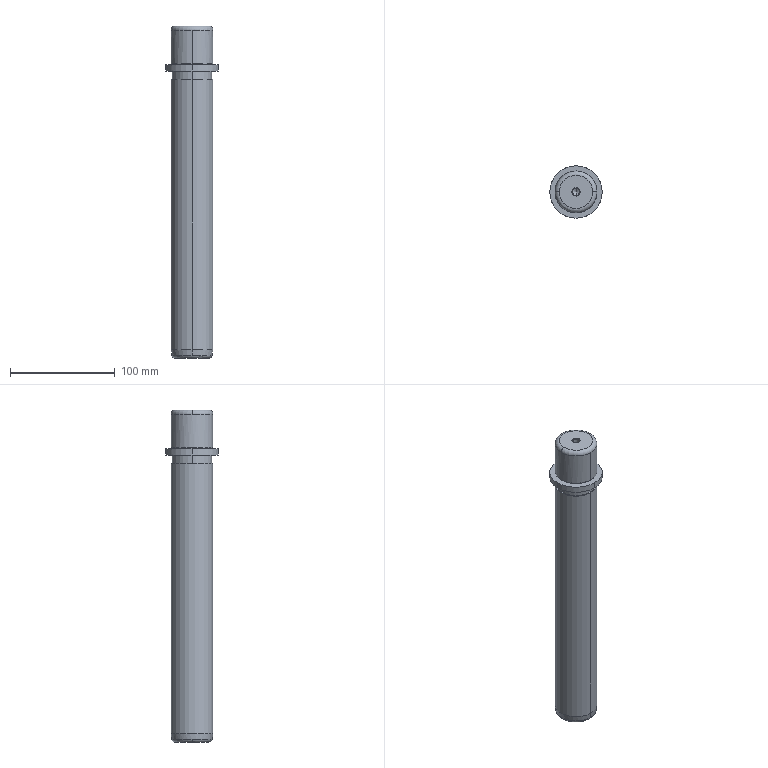Part | CATIA | 1 solid | 37 faces | box 50 x 50 x 317 mm | volume 398728 mm3 | cylinder 19 | cone 8 | plane 6 | torus 4 | commonest cylinder face diameters 38 x7 6.647 x4 40 x4 50 x4
STEP:
#1=CARTESIAN_POINT('',(0.,-3.323,16.609));
#2=VERTEX_POINT('',#1);
#3=CARTESIAN_POINT('',(0.,0.,14.691));
#4=VERTEX_POINT('',#3);
#5=CARTESIAN_POINT('',(0.,-433013.533,250015.17));
#6=DIRECTION('',(0.,-0.866,0.5));
#7=VECTOR('',#6,1.);
#8=LINE('',#5,#7);
#9=EDGE_CURVE('',#2,#4,#8,.F.);
#10=ORIENTED_EDGE('',*,*,#9,.T.);
#11=CARTESIAN_POINT('',(0.,3.323,16.609));
#12=VERTEX_POINT('',#11);
#13=CARTESIAN_POINT('',(0.,433013.533,250015.17));
#14=DIRECTION('',(0.,0.866,0.5));
#15=VECTOR('',#14,1.);
#16=LINE('',#13,#15);
#17=EDGE_CURVE('',#4,#12,#16,.T.);
#18=ORIENTED_EDGE('',*,*,#17,.T.);
#19=CARTESIAN_POINT('',(0.,0.,16.609));
#20=DIRECTION('',(0.,0.,1.));
#21=AXIS2_PLACEMENT_3D('',#19,#20,$);
#22=CIRCLE('',#21,3.323);
#23=EDGE_CURVE('',#12,#2,#22,.T.);
#24=ORIENTED_EDGE('',*,*,#23,.T.);
#25=EDGE_LOOP('',(#10,#18,#24));
#26=FACE_OUTER_BOUND('',#25,.T.);
#27=CARTESIAN_POINT('',(0.,0.,15.65));
#28=DIRECTION('',(0.,0.,1.));
#29=DIRECTION('',(0.,1.,0.));
#30=AXIS2_PLACEMENT_3D('',#27,#28,#29);
#31=CONICAL_SURFACE('',#30,1.662,1.047);
#32=ADVANCED_FACE('',(#26),#31,.F.);
#33=ORIENTED_EDGE('',*,*,#9,.F.);
#34=CARTESIAN_POINT('',(0.,0.,16.609));
#35=DIRECTION('',(0.,0.,1.));
#36=AXIS2_PLACEMENT_3D('',#34,#35,$);
#37=CIRCLE('',#36,3.323);
#38=EDGE_CURVE('',#2,#12,#37,.T.);
#39=ORIENTED_EDGE('',*,*,#38,.T.);
#40=ORIENTED_EDGE('',*,*,#17,.F.);
#41=EDGE_LOOP('',(#33,#39,#40));
#42=FACE_OUTER_BOUND('',#41,.T.);
#43=CARTESIAN_POINT('',(0.,0.,15.65));
#44=DIRECTION('',(0.,0.,1.));
#45=DIRECTION('',(0.,-1.,0.));
#46=AXIS2_PLACEMENT_3D('',#43,#44,#45);
#47=CONICAL_SURFACE('',#46,1.662,1.047);
#48=ADVANCED_FACE('',(#42),#47,.F.);
#49=CARTESIAN_POINT('',(0.,3.324,36.324));
#50=VERTEX_POINT('',#49);
#51=CARTESIAN_POINT('',(0.,3.324,26.466));
#52=DIRECTION('',(0.,0.,-1.));
#53=VECTOR('',#52,1.);
#54=LINE('',#51,#53);
#55=EDGE_CURVE('',#12,#50,#54,.F.);
#56=ORIENTED_EDGE('',*,*,#55,.T.);
#57=CARTESIAN_POINT('',(0.,-3.324,36.324));
#58=VERTEX_POINT('',#57);
#59=CARTESIAN_POINT('',(0.,0.,36.324));
#60=DIRECTION('',(0.,0.,-1.));
#61=AXIS2_PLACEMENT_3D('',#59,#60,$);
#62=CIRCLE('',#61,3.324);
#63=EDGE_CURVE('',#50,#58,#62,.F.);
#64=ORIENTED_EDGE('',*,*,#63,.T.);
#65=CARTESIAN_POINT('',(0.,-3.324,26.466));
#66=DIRECTION('',(0.,0.,-1.));
#67=VECTOR('',#66,1.);
#68=LINE('',#65,#67);
#69=EDGE_CURVE('',#58,#2,#68,.T.);
#70=ORIENTED_EDGE('',*,*,#69,.T.);
#71=ORIENTED_EDGE('',*,*,#23,.F.);
#72=EDGE_LOOP('',(#56,#64,#70,#71));
#73=FACE_OUTER_BOUND('',#72,.T.);
#74=CARTESIAN_POINT('',(0.,0.,26.466));
#75=DIRECTION('',(0.,0.,-1.));
#76=DIRECTION('',(0.,-1.,0.));
#77=AXIS2_PLACEMENT_3D('',#74,#75,#76);
#78=CYLINDRICAL_SURFACE('',#77,3.324);
#79=ADVANCED_FACE('',(#73),#78,.F.);
#80=ORIENTED_EDGE('',*,*,#55,.F.);
#81=ORIENTED_EDGE('',*,*,#38,.F.);
#82=ORIENTED_EDGE('',*,*,#69,.F.);
#83=CARTESIAN_POINT('',(0.,0.,36.324));
#84=DIRECTION('',(0.,0.,-1.));
#85=AXIS2_PLACEMENT_3D('',#83,#84,$);
#86=CIRCLE('',#85,3.324);
#87=EDGE_CURVE('',#58,#50,#86,.F.);
#88=ORIENTED_EDGE('',*,*,#87,.T.);
#89=EDGE_LOOP('',(#80,#81,#82,#88));
#90=FACE_OUTER_BOUND('',#89,.T.);
#91=CARTESIAN_POINT('',(0.,0.,26.466));
#92=DIRECTION('',(0.,0.,-1.));
#93=DIRECTION('',(0.,1.,0.));
#94=AXIS2_PLACEMENT_3D('',#91,#92,#93);
#95=CYLINDRICAL_SURFACE('',#94,3.324);
#96=ADVANCED_FACE('',(#90),#95,.F.);
#97=CARTESIAN_POINT('',(0.,4.,37.));
#98=VERTEX_POINT('',#97);
#99=CARTESIAN_POINT('',(0.,353555.221,353588.221));
#100=DIRECTION('',(0.,0.7071,0.7071));
#101=VECTOR('',#100,1.);
#102=LINE('',#99,#101);
#103=EDGE_CURVE('',#50,#98,#102,.T.);
#104=ORIENTED_EDGE('',*,*,#103,.T.);
#105=CARTESIAN_POINT('',(0.,-4.,37.));
#106=VERTEX_POINT('',#105);
#107=CARTESIAN_POINT('',(0.,0.,37.));
#108=DIRECTION('',(0.,0.,1.));
#109=AXIS2_PLACEMENT_3D('',#107,#108,$);
#110=CIRCLE('',#109,4.);
#111=EDGE_CURVE('',#98,#106,#110,.T.);
#112=ORIENTED_EDGE('',*,*,#111,.T.);
#113=CARTESIAN_POINT('',(0.,-353555.221,353588.221));
#114=DIRECTION('',(0.,-0.7071,0.7071));
#115=VECTOR('',#114,1.);
#116=LINE('',#113,#115);
#117=EDGE_CURVE('',#106,#58,#116,.F.);
#118=ORIENTED_EDGE('',*,*,#117,.T.);
#119=ORIENTED_EDGE('',*,*,#63,.F.);
#120=EDGE_LOOP('',(#104,#112,#118,#119));
#121=FACE_OUTER_BOUND('',#120,.T.);
#122=CARTESIAN_POINT('',(0.,0.,36.662));
#123=DIRECTION('',(0.,0.,1.));
#124=DIRECTION('',(0.,1.,0.));
#125=AXIS2_PLACEMENT_3D('',#122,#123,#124);
#126=CONICAL_SURFACE('',#125,3.662,0.7854);
#127=ADVANCED_FACE('',(#121),#126,.F.);
#128=ORIENTED_EDGE('',*,*,#103,.F.);
#129=ORIENTED_EDGE('',*,*,#87,.F.);
#130=ORIENTED_EDGE('',*,*,#117,.F.);
#131=CARTESIAN_POINT('',(0.,0.,37.));
#132=DIRECTION('',(0.,0.,1.));
#133=AXIS2_PLACEMENT_3D('',#131,#132,$);
#134=CIRCLE('',#133,4.);
#135=EDGE_CURVE('',#106,#98,#134,.T.);
#136=ORIENTED_EDGE('',*,*,#135,.T.);
#137=EDGE_LOOP('',(#128,#129,#130,#136));
#138=FACE_OUTER_BOUND('',#137,.T.);
#139=CARTESIAN_POINT('',(0.,0.,36.662));
#140=DIRECTION('',(0.,0.,1.));
#141=DIRECTION('',(0.,-1.,0.));
#142=AXIS2_PLACEMENT_3D('',#139,#140,#141);
#143=CONICAL_SURFACE('',#142,3.662,0.7854);
#144=ADVANCED_FACE('',(#138),#143,.F.);
#145=CARTESIAN_POINT('',(0.,16.,37.));
#146=VERTEX_POINT('',#145);
#147=CARTESIAN_POINT('',(-16.,0.,37.));
#148=VERTEX_POINT('',#147);
#149=CARTESIAN_POINT('',(0.,0.,37.));
#150=DIRECTION('',(0.,0.,1.));
#151=AXIS2_PLACEMENT_3D('',#149,#150,$);
#152=CIRCLE('',#151,16.);
#153=EDGE_CURVE('',#146,#148,#152,.T.);
#154=ORIENTED_EDGE('',*,*,#153,.T.);
#155=CARTESIAN_POINT('',(16.,0.,37.));
#156=VERTEX_POINT('',#155);
#157=CARTESIAN_POINT('',(0.,0.,37.));
#158=DIRECTION('',(0.,0.,1.));
#159=AXIS2_PLACEMENT_3D('',#157,#158,$);
#160=CIRCLE('',#159,16.);
#161=EDGE_CURVE('',#148,#156,#160,.T.);
#162=ORIENTED_EDGE('',*,*,#161,.T.);
#163=CARTESIAN_POINT('',(0.,0.,37.));
#164=DIRECTION('',(0.,0.,1.));
#165=AXIS2_PLACEMENT_3D('',#163,#164,$);
#166=CIRCLE('',#165,16.);
#167=EDGE_CURVE('',#156,#146,#166,.T.);
#168=ORIENTED_EDGE('',*,*,#167,.T.);
#169=EDGE_LOOP('',(#154,#162,#168));
#170=FACE_OUTER_BOUND('',#169,.T.);
#171=ORIENTED_EDGE('',*,*,#111,.F.);
#172=ORIENTED_EDGE('',*,*,#135,.F.);
#173=EDGE_LOOP('',(#171,#172));
#174=FACE_BOUND('',#173,.T.);
#175=CARTESIAN_POINT('',(0.,10.,37.));
#176=DIRECTION('',(0.,0.,1.));
#177=DIRECTION('',(0.,1.,0.));
#178=AXIS2_PLACEMENT_3D('',#175,#176,#177);
#179=PLANE('',#178);
#180=ADVANCED_FACE('',(#170,#174),#179,.T.);
#181=CARTESIAN_POINT('',(20.,0.,33.));
#182=VERTEX_POINT('',#181);
#183=CARTESIAN_POINT('',(16.,0.,33.));
#184=DIRECTION('',(0.,-1.,0.));
#185=AXIS2_PLACEMENT_3D('',#183,#184,$);
#186=CIRCLE('',#185,4.);
#187=EDGE_CURVE('',#182,#156,#186,.T.);
#188=ORIENTED_EDGE('',*,*,#187,.F.);
#189=CARTESIAN_POINT('',(0.,20.,33.));
#190=VERTEX_POINT('',#189);
#191=CARTESIAN_POINT('',(0.,0.,33.));
#192=DIRECTION('',(0.,0.,1.));
#193=AXIS2_PLACEMENT_3D('',#191,#192,$);
#194=CIRCLE('',#193,20.);
#195=EDGE_CURVE('',#182,#190,#194,.T.);
#196=ORIENTED_EDGE('',*,*,#195,.T.);
#197=CARTESIAN_POINT('',(-20.,0.,33.));
#198=VERTEX_POINT('',#197);
#199=CARTESIAN_POINT('',(0.,0.,33.));
#200=DIRECTION('',(0.,0.,1.));
#201=AXIS2_PLACEMENT_3D('',#199,#200,$);
#202=CIRCLE('',#201,20.);
#203=EDGE_CURVE('',#190,#198,#202,.T.);
#204=ORIENTED_EDGE('',*,*,#203,.T.);
#205=CARTESIAN_POINT('',(-16.,0.,33.));
#206=DIRECTION('',(0.,1.,0.));
#207=AXIS2_PLACEMENT_3D('',#205,#206,$);
#208=CIRCLE('',#207,4.);
#209=EDGE_CURVE('',#148,#198,#208,.F.);
#210=ORIENTED_EDGE('',*,*,#209,.F.);
#211=ORIENTED_EDGE('',*,*,#153,.F.);
#212=ORIENTED_EDGE('',*,*,#167,.F.);
#213=EDGE_LOOP('',(#188,#196,#204,#210,#211,#212));
#214=FACE_OUTER_BOUND('',#213,.T.);
#215=CARTESIAN_POINT('',(0.,0.,33.));
#216=DIRECTION('',(0.,0.,1.));
#217=DIRECTION('',(1.,0.,0.));
#218=AXIS2_PLACEMENT_3D('',#215,#216,#217);
#219=TOROIDAL_SURFACE('',#218,16.,4.);
#220=ADVANCED_FACE('',(#214),#219,.T.);
#221=ORIENTED_EDGE('',*,*,#187,.T.);
#222=ORIENTED_EDGE('',*,*,#161,.F.);
#223=ORIENTED_EDGE('',*,*,#209,.T.);
#224=CARTESIAN_POINT('',(0.,-20.,33.));
#225=VERTEX_POINT('',#224);
#226=CARTESIAN_POINT('',(0.,0.,33.));
#227=DIRECTION('',(0.,0.,1.));
#228=AXIS2_PLACEMENT_3D('',#226,#227,$);
#229=CIRCLE('',#228,20.);
#230=EDGE_CURVE('',#198,#225,#229,.T.);
#231=ORIENTED_EDGE('',*,*,#230,.T.);
#232=CARTESIAN_POINT('',(0.,0.,33.));
#233=DIRECTION('',(0.,0.,1.));
#234=AXIS2_PLACEMENT_3D('',#232,#233,$);
#235=CIRCLE('',#234,20.);
#236=EDGE_CURVE('',#225,#182,#235,.T.);
#237=ORIENTED_EDGE('',*,*,#236,.T.);
#238=EDGE_LOOP('',(#221,#222,#223,#231,#237));
#239=FACE_OUTER_BOUND('',#238,.T.);
#240=CARTESIAN_POINT('',(0.,0.,33.));
#241=DIRECTION('',(0.,0.,1.));
#242=DIRECTION('',(-1.,0.,0.));
#243=AXIS2_PLACEMENT_3D('',#240,#241,#242);
#244=TOROIDAL_SURFACE('',#243,16.,4.);
#245=ADVANCED_FACE('',(#239),#244,.T.);
#246=CARTESIAN_POINT('',(0.,20.,1.));
#247=VERTEX_POINT('',#246);
#248=CARTESIAN_POINT('',(0.,20.,17.));
#249=DIRECTION('',(0.,0.,-1.));
#250=VECTOR('',#249,1.);
#251=LINE('',#248,#250);
#252=EDGE_CURVE('',#247,#190,#251,.F.);
#253=ORIENTED_EDGE('',*,*,#252,.T.);
#254=ORIENTED_EDGE('',*,*,#195,.F.);
#255=ORIENTED_EDGE('',*,*,#236,.F.);
#256=CARTESIAN_POINT('',(0.,-20.,1.));
#257=VERTEX_POINT('',#256);
#258=CARTESIAN_POINT('',(0.,-20.,17.));
#259=DIRECTION('',(0.,0.,-1.));
#260=VECTOR('',#259,1.);
#261=LINE('',#258,#260);
#262=EDGE_CURVE('',#225,#257,#261,.T.);
#263=ORIENTED_EDGE('',*,*,#262,.T.);
#264=CARTESIAN_POINT('',(0.,0.,1.));
#265=DIRECTION('',(0.,0.,-1.));
#266=AXIS2_PLACEMENT_3D('',#264,#265,$);
#267=CIRCLE('',#266,20.);
#268=EDGE_CURVE('',#257,#247,#267,.F.);
#269=ORIENTED_EDGE('',*,*,#268,.T.);
#270=EDGE_LOOP('',(#253,#254,#255,#263,#269));
#271=FACE_OUTER_BOUND('',#270,.T.);
#272=CARTESIAN_POINT('',(0.,0.,17.));
#273=DIRECTION('',(0.,0.,-1.));
#274=DIRECTION('',(0.,1.,0.));
#275=AXIS2_PLACEMENT_3D('',#272,#273,#274);
#276=CYLINDRICAL_SURFACE('',#275,20.);
#277=ADVANCED_FACE('',(#271),#276,.T.);
#278=ORIENTED_EDGE('',*,*,#252,.F.);
#279=CARTESIAN_POINT('',(0.,0.,1.));
#280=DIRECTION('',(0.,0.,-1.));
#281=AXIS2_PLACEMENT_3D('',#279,#280,$);
#282=CIRCLE('',#281,20.);
#283=EDGE_CURVE('',#247,#257,#282,.F.);
#284=ORIENTED_EDGE('',*,*,#283,.T.);
#285=ORIENTED_EDGE('',*,*,#262,.F.);
#286=ORIENTED_EDGE('',*,*,#230,.F.);
#287=ORIENTED_EDGE('',*,*,#203,.F.);
#288=EDGE_LOOP('',(#278,#284,#285,#286,#287));
#289=FACE_OUTER_BOUND('',#288,.T.);
#290=CARTESIAN_POINT('',(0.,0.,17.));
#291=DIRECTION('',(0.,0.,-1.));
#292=DIRECTION('',(0.,-1.,0.));
#293=AXIS2_PLACEMENT_3D('',#290,#291,#292);
#294=CYLINDRICAL_SURFACE('',#293,20.);
#295=ADVANCED_FACE('',(#289),#294,.T.);
#296=ORIENTED_EDGE('',*,*,#283,.F.);
#297=ORIENTED_EDGE('',*,*,#268,.F.);
#298=EDGE_LOOP('',(#296,#297));
#299=FACE_OUTER_BOUND('',#298,.T.);
#300=CARTESIAN_POINT('',(0.,19.,1.));
#301=VERTEX_POINT('',#300);
#302=CARTESIAN_POINT('',(-19.,0.,1.));
#303=VERTEX_POINT('',#302);
#304=CARTESIAN_POINT('',(0.,19.,1.));
#305=CARTESIAN_POINT('',(-1.922,19.,1.));
#306=CARTESIAN_POINT('',(-3.844,18.757,1.));
#307=CARTESIAN_POINT('',(-5.725,18.271,1.));
#308=CARTESIAN_POINT('',(-9.323,16.834,1.));
#309=CARTESIAN_POINT('',(-12.45,14.547,1.));
#310=CARTESIAN_POINT('',(-13.86,13.21,1.));
#311=CARTESIAN_POINT('',(-16.311,10.21,1.));
#312=CARTESIAN_POINT('',(-17.938,6.694,1.));
#313=CARTESIAN_POINT('',(-18.524,4.842,1.));
#314=CARTESIAN_POINT('',(-18.907,2.734,1.));
#315=CARTESIAN_POINT('',(-18.992,0.6103,1.));
#316=CARTESIAN_POINT('',(-18.997,0.4069,1.));
#317=CARTESIAN_POINT('',(-19.,0.2034,1.));
#318=CARTESIAN_POINT('',(-19.,0.,1.));
#319=B_SPLINE_CURVE_WITH_KNOTS('',5,(#304,#305,#306,#307,#308,#309,#310,#311,#312,#313,#314,#315,#316,#317,#318),.UNSPECIFIED.,.F.,.U.,(6,3,3,3,6),(0.,13.624,27.249,40.873,42.316),.UNSPECIFIED.);
#320=EDGE_CURVE('',#301,#303,#319,.T.);
#321=ORIENTED_EDGE('',*,*,#320,.T.);
#322=CARTESIAN_POINT('',(0.,-19.,1.));
#323=VERTEX_POINT('',#322);
#324=CARTESIAN_POINT('',(-19.,0.,1.));
#325=CARTESIAN_POINT('',(-19.,-1.718,1.));
#326=CARTESIAN_POINT('',(-18.806,-3.437,1.));
#327=CARTESIAN_POINT('',(-18.417,-5.126,1.));
#328=CARTESIAN_POINT('',(-17.197,-8.58,1.));
#329=CARTESIAN_POINT('',(-15.192,-11.653,1.));
#330=CARTESIAN_POINT('',(-13.933,-13.133,1.));
#331=CARTESIAN_POINT('',(-11.068,-15.741,1.));
#332=CARTESIAN_POINT('',(-7.645,-17.554,1.));
#333=CARTESIAN_POINT('',(-5.826,-18.239,1.));
#334=CARTESIAN_POINT('',(-3.542,-18.78,1.));
#335=CARTESIAN_POINT('',(-1.221,-18.967,1.));
#336=CARTESIAN_POINT('',(-0.8135,-18.989,1.));
#337=CARTESIAN_POINT('',(-0.4067,-19.,1.));
#338=CARTESIAN_POINT('',(0.,-19.,1.));
#339=B_SPLINE_CURVE_WITH_KNOTS('',5,(#324,#325,#326,#327,#328,#329,#330,#331,#332,#333,#334,#335,#336,#337,#338),.UNSPECIFIED.,.F.,.U.,(6,3,3,3,6),(42.316,54.498,68.122,81.747,84.63),.UNSPECIFIED.);
#340=EDGE_CURVE('',#303,#323,#339,.T.);
#341=ORIENTED_EDGE('',*,*,#340,.T.);
#342=CARTESIAN_POINT('',(0.,-19.,1.));
#343=CARTESIAN_POINT('',(1.922,-19.,1.));
#344=CARTESIAN_POINT('',(3.844,-18.757,1.));
#345=CARTESIAN_POINT('',(5.725,-18.271,1.));
#346=CARTESIAN_POINT('',(9.323,-16.834,1.));
#347=CARTESIAN_POINT('',(12.45,-14.547,1.));
#348=CARTESIAN_POINT('',(13.86,-13.21,1.));
#349=CARTESIAN_POINT('',(16.311,-10.21,1.));
#350=CARTESIAN_POINT('',(17.938,-6.694,1.));
#351=CARTESIAN_POINT('',(18.524,-4.842,1.));
#352=CARTESIAN_POINT('',(19.215,-1.03,1.));
#353=CARTESIAN_POINT('',(18.936,2.834,1.));
#354=CARTESIAN_POINT('',(18.551,4.739,1.));
#355=CARTESIAN_POINT('',(17.309,8.408,1.));
#356=CARTESIAN_POINT('',(15.192,11.653,1.));
#357=CARTESIAN_POINT('',(13.933,13.133,1.));
#358=CARTESIAN_POINT('',(11.068,15.741,1.));
#359=CARTESIAN_POINT('',(7.645,17.554,1.));
#360=CARTESIAN_POINT('',(5.826,18.239,1.));
#361=CARTESIAN_POINT('',(3.542,18.78,1.));
#362=CARTESIAN_POINT('',(1.221,18.967,1.));
#363=CARTESIAN_POINT('',(0.8135,18.989,1.));
#364=CARTESIAN_POINT('',(0.4067,19.,1.));
#365=CARTESIAN_POINT('',(0.,19.,1.));
#366=B_SPLINE_CURVE_WITH_KNOTS('',5,(#342,#343,#344,#345,#346,#347,#348,#349,#350,#351,#352,#353,#354,#355,#356,#357,#358,#359,#360,#361,#362,#363,#364,#365),.UNSPECIFIED.,.F.,.U.,(6,3,3,3,3,3,3,6),(0.,13.624,27.249,40.873,54.498,68.122,81.747,84.63),.UNSPECIFIED.);
#367=EDGE_CURVE('',#323,#301,#366,.T.);
#368=ORIENTED_EDGE('',*,*,#367,.T.);
#369=EDGE_LOOP('',(#321,#341,#368));
#370=FACE_BOUND('',#369,.T.);
#371=CARTESIAN_POINT('',(0.,19.5,1.));
#372=DIRECTION('',(0.,0.,-1.));
#373=DIRECTION('',(0.,-1.,0.));
#374=AXIS2_PLACEMENT_3D('',#371,#372,#373);
#375=PLANE('',#374);
#376=ADVANCED_FACE('',(#299,#370),#375,.T.);
#377=CARTESIAN_POINT('',(-19.,0.,0.));
#378=VERTEX_POINT('',#377);
#379=CARTESIAN_POINT('',(-19.,0.,0.5));
#380=DIRECTION('',(0.,0.,-1.));
#381=VECTOR('',#380,1.);
#382=LINE('',#379,#381);
#383=EDGE_CURVE('',#303,#378,#382,.T.);
#384=ORIENTED_EDGE('',*,*,#383,.F.);
#385=ORIENTED_EDGE('',*,*,#320,.F.);
#386=CARTESIAN_POINT('',(0.,19.,0.));
#387=VERTEX_POINT('',#386);
#388=CARTESIAN_POINT('',(0.,19.,0.5));
#389=DIRECTION('',(0.,0.,-1.));
#390=VECTOR('',#389,1.);
#391=LINE('',#388,#390);
#392=EDGE_CURVE('',#387,#301,#391,.F.);
#393=ORIENTED_EDGE('',*,*,#392,.F.);
#394=CARTESIAN_POINT('',(0.,0.,0.));
#395=DIRECTION('',(0.,0.,-1.));
#396=AXIS2_PLACEMENT_3D('',#394,#395,$);
#397=CIRCLE('',#396,19.);
#398=EDGE_CURVE('',#387,#378,#397,.F.);
#399=ORIENTED_EDGE('',*,*,#398,.T.);
#400=EDGE_LOOP('',(#384,#385,#393,#399));
#401=FACE_OUTER_BOUND('',#400,.T.);
#402=CARTESIAN_POINT('',(0.,0.,0.5));
#403=DIRECTION('',(0.,0.,-1.));
#404=DIRECTION('',(-1.,0.,0.));
#405=AXIS2_PLACEMENT_3D('',#402,#403,#404);
#406=CYLINDRICAL_SURFACE('',#405,19.);
#407=ADVANCED_FACE('',(#401),#406,.T.);
#408=ORIENTED_EDGE('',*,*,#383,.T.);
#409=CARTESIAN_POINT('',(0.,-19.,0.));
#410=VERTEX_POINT('',#409);
#411=CARTESIAN_POINT('',(0.,0.,0.));
#412=DIRECTION('',(0.,0.,-1.));
#413=AXIS2_PLACEMENT_3D('',#411,#412,$);
#414=CIRCLE('',#413,19.);
#415=EDGE_CURVE('',#378,#410,#414,.F.);
#416=ORIENTED_EDGE('',*,*,#415,.T.);
#417=CARTESIAN_POINT('',(0.,-19.,0.5));
#418=DIRECTION('',(0.,0.,-1.));
#419=VECTOR('',#418,1.);
#420=LINE('',#417,#419);
#421=EDGE_CURVE('',#323,#410,#420,.T.);
#422=ORIENTED_EDGE('',*,*,#421,.F.);
#423=ORIENTED_EDGE('',*,*,#340,.F.);
#424=EDGE_LOOP('',(#408,#416,#422,#423));
#425=FACE_OUTER_BOUND('',#424,.T.);
#426=CARTESIAN_POINT('',(0.,0.,0.5));
#427=DIRECTION('',(0.,0.,-1.));
#428=DIRECTION('',(1.,0.,0.));
#429=AXIS2_PLACEMENT_3D('',#426,#427,#428);
#430=CYLINDRICAL_SURFACE('',#429,19.);
#431=ADVANCED_FACE('',(#425),#430,.T.);
#432=ORIENTED_EDGE('',*,*,#392,.T.);
#433=ORIENTED_EDGE('',*,*,#367,.F.);
#434=ORIENTED_EDGE('',*,*,#421,.T.);
#435=CARTESIAN_POINT('',(0.,0.,0.));
#436=DIRECTION('',(0.,0.,-1.));
#437=AXIS2_PLACEMENT_3D('',#435,#436,$);
#438=CIRCLE('',#437,19.);
#439=EDGE_CURVE('',#410,#387,#438,.F.);
#440=ORIENTED_EDGE('',*,*,#439,.T.);
#441=EDGE_LOOP('',(#432,#433,#434,#440));
#442=FACE_OUTER_BOUND('',#441,.T.);
#443=CARTESIAN_POINT('',(0.,0.,0.5));
#444=DIRECTION('',(0.,0.,-1.));
#445=DIRECTION('',(0.,1.,0.));
#446=AXIS2_PLACEMENT_3D('',#443,#444,#445);
#447=CYLINDRICAL_SURFACE('',#446,19.);
#448=ADVANCED_FACE('',(#442),#447,.T.);
#449=CARTESIAN_POINT('',(0.,25.,0.));
#450=VERTEX_POINT('',#449);
#451=CARTESIAN_POINT('',(-25.,0.,0.));
#452=VERTEX_POINT('',#451);
#453=CARTESIAN_POINT('',(0.000000003,-0.000000003,0.));
#454=DIRECTION('',(0.,0.,1.));
#455=AXIS2_PLACEMENT_3D('',#453,#454,$);
#456=CIRCLE('',#455,25.);
#457=EDGE_CURVE('',#450,#452,#456,.T.);
#458=ORIENTED_EDGE('',*,*,#457,.T.);
#459=CARTESIAN_POINT('',(0.,-25.,0.));
#460=VERTEX_POINT('',#459);
#461=CARTESIAN_POINT('',(0.000000003,0.000000003,0.));
#462=DIRECTION('',(0.,0.,1.));
#463=AXIS2_PLACEMENT_3D('',#461,#462,$);
#464=CIRCLE('',#463,25.);
#465=EDGE_CURVE('',#452,#460,#464,.T.);
#466=ORIENTED_EDGE('',*,*,#465,.T.);
#467=CARTESIAN_POINT('',(25.,0.,0.));
#468=VERTEX_POINT('',#467);
#469=CARTESIAN_POINT('',(-0.000000003,0.000000003,0.));
#470=DIRECTION('',(0.,0.,1.));
#471=AXIS2_PLACEMENT_3D('',#469,#470,$);
#472=CIRCLE('',#471,25.);
#473=EDGE_CURVE('',#468,#460,#472,.F.);
#474=ORIENTED_EDGE('',*,*,#473,.F.);
#475=CARTESIAN_POINT('',(-0.000000003,-0.000000003,0.));
#476=DIRECTION('',(0.,0.,1.));
#477=AXIS2_PLACEMENT_3D('',#475,#476,$);
#478=CIRCLE('',#477,25.);
#479=EDGE_CURVE('',#450,#468,#478,.F.);
#480=ORIENTED_EDGE('',*,*,#479,.F.);
#481=EDGE_LOOP('',(#458,#466,#474,#480));
#482=FACE_OUTER_BOUND('',#481,.T.);
#483=ORIENTED_EDGE('',*,*,#415,.F.);
#484=ORIENTED_EDGE('',*,*,#398,.F.);
#485=ORIENTED_EDGE('',*,*,#439,.F.);
#486=EDGE_LOOP('',(#483,#484,#485));
#487=FACE_BOUND('',#486,.T.);
#488=CARTESIAN_POINT('',(0.,22.,0.));
#489=DIRECTION('',(0.,0.,1.));
#490=DIRECTION('',(0.,1.,0.));
#491=AXIS2_PLACEMENT_3D('',#488,#489,#490);
#492=PLANE('',#491);
#493=ADVANCED_FACE('',(#482,#487),#492,.T.);
#494=CARTESIAN_POINT('',(-19.671,15.429,-6.));
#495=VERTEX_POINT('',#494);
#496=CARTESIAN_POINT('',(-25.,0.,-6.));
#497=VERTEX_POINT('',#496);
#498=CARTESIAN_POINT('',(0.,0.,-6.));
#499=DIRECTION('',(0.,0.,-1.));
#500=AXIS2_PLACEMENT_3D('',#498,#499,$);
#501=CIRCLE('',#500,25.);
#502=EDGE_CURVE('',#495,#497,#501,.F.);
#503=ORIENTED_EDGE('',*,*,#502,.T.);
#504=CARTESIAN_POINT('',(-25.,0.,-3.));
#505=DIRECTION('',(0.,0.,-1.));
#506=VECTOR('',#505,1.);
#507=LINE('',#504,#506);
#508=EDGE_CURVE('',#497,#452,#507,.F.);
#509=ORIENTED_EDGE('',*,*,#508,.T.);
#510=ORIENTED_EDGE('',*,*,#457,.F.);
#511=CARTESIAN_POINT('',(0.,25.,-6.));
#512=VERTEX_POINT('',#511);
#513=CARTESIAN_POINT('',(0.,25.,-3.));
#514=DIRECTION('',(0.,0.,-1.));
#515=VECTOR('',#514,1.);
#516=LINE('',#513,#515);
#517=EDGE_CURVE('',#512,#450,#516,.F.);
#518=ORIENTED_EDGE('',*,*,#517,.F.);
#519=CARTESIAN_POINT('',(-15.429,19.671,-6.));
#520=VERTEX_POINT('',#519);
#521=CARTESIAN_POINT('',(0.,0.,-6.));
#522=DIRECTION('',(0.,0.,-1.));
#523=AXIS2_PLACEMENT_3D('',#521,#522,$);
#524=CIRCLE('',#523,25.);
#525=EDGE_CURVE('',#512,#520,#524,.F.);
#526=ORIENTED_EDGE('',*,*,#525,.T.);
#527=CARTESIAN_POINT('',(0.,0.,-6.));
#528=DIRECTION('',(0.,0.,-1.));
#529=AXIS2_PLACEMENT_3D('',#527,#528,$);
#530=CIRCLE('',#529,25.);
#531=EDGE_CURVE('',#495,#520,#530,.T.);
#532=ORIENTED_EDGE('',*,*,#531,.F.);
#533=EDGE_LOOP('',(#503,#509,#510,#518,#526,#532));
#534=FACE_OUTER_BOUND('',#533,.T.);
#535=CARTESIAN_POINT('',(0.,0.,-3.));
#536=DIRECTION('',(0.,0.,-1.));
#537=DIRECTION('',(-1.,0.,0.));
#538=AXIS2_PLACEMENT_3D('',#535,#536,#537);
#539=CYLINDRICAL_SURFACE('',#538,25.);
#540=ADVANCED_FACE('',(#534),#539,.T.);
#541=CARTESIAN_POINT('',(-15.429,-19.671,-6.));
#542=VERTEX_POINT('',#541);
#543=CARTESIAN_POINT('',(0.,-25.,-6.));
#544=VERTEX_POINT('',#543);
#545=CARTESIAN_POINT('',(0.,0.,-6.));
#546=DIRECTION('',(0.,0.,-1.));
#547=AXIS2_PLACEMENT_3D('',#545,#546,$);
#548=CIRCLE('',#547,25.);
#549=EDGE_CURVE('',#542,#544,#548,.F.);
#550=ORIENTED_EDGE('',*,*,#549,.T.);
#551=CARTESIAN_POINT('',(0.,-25.,-3.));
#552=DIRECTION('',(0.,0.,-1.));
#553=VECTOR('',#552,1.);
#554=LINE('',#551,#553);
#555=EDGE_CURVE('',#460,#544,#554,.T.);
#556=ORIENTED_EDGE('',*,*,#555,.F.);
#557=ORIENTED_EDGE('',*,*,#465,.F.);
#558=ORIENTED_EDGE('',*,*,#508,.F.);
#559=CARTESIAN_POINT('',(-19.671,-15.429,-6.));
#560=VERTEX_POINT('',#559);
#561=CARTESIAN_POINT('',(0.,0.,-6.));
#562=DIRECTION('',(0.,0.,-1.));
#563=AXIS2_PLACEMENT_3D('',#561,#562,$);
#564=CIRCLE('',#563,25.);
#565=EDGE_CURVE('',#497,#560,#564,.F.);
#566=ORIENTED_EDGE('',*,*,#565,.T.);
#567=CARTESIAN_POINT('',(0.,0.,-6.));
#568=DIRECTION('',(0.,0.,-1.));
#569=AXIS2_PLACEMENT_3D('',#567,#568,$);
#570=CIRCLE('',#569,25.);
#571=EDGE_CURVE('',#542,#560,#570,.T.);
#572=ORIENTED_EDGE('',*,*,#571,.F.);
#573=EDGE_LOOP('',(#550,#556,#557,#558,#566,#572));
#574=FACE_OUTER_BOUND('',#573,.T.);
#575=CARTESIAN_POINT('',(0.,0.,-3.));
#576=DIRECTION('',(0.,0.,-1.));
#577=DIRECTION('',(1.,0.,0.));
#578=AXIS2_PLACEMENT_3D('',#575,#576,#577);
#579=CYLINDRICAL_SURFACE('',#578,25.);
#580=ADVANCED_FACE('',(#574),#579,.T.);
#581=CARTESIAN_POINT('',(25.,0.,-6.));
#582=VERTEX_POINT('',#581);
#583=CARTESIAN_POINT('',(19.671,-15.429,-6.));
#584=VERTEX_POINT('',#583);
#585=CARTESIAN_POINT('',(0.,0.,-6.));
#586=DIRECTION('',(0.,0.,-1.));
#587=AXIS2_PLACEMENT_3D('',#585,#586,$);
#588=CIRCLE('',#587,25.);
#589=EDGE_CURVE('',#582,#584,#588,.T.);
#590=ORIENTED_EDGE('',*,*,#589,.F.);
#591=CARTESIAN_POINT('',(25.,0.,-3.));
#592=DIRECTION('',(0.,0.,-1.));
#593=VECTOR('',#592,1.);
#594=LINE('',#591,#593);
#595=EDGE_CURVE('',#468,#582,#594,.T.);
#596=ORIENTED_EDGE('',*,*,#595,.F.);
#597=ORIENTED_EDGE('',*,*,#473,.T.);
#598=ORIENTED_EDGE('',*,*,#555,.T.);
#599=CARTESIAN_POINT('',(15.429,-19.671,-6.));
#600=VERTEX_POINT('',#599);
#601=CARTESIAN_POINT('',(0.,0.,-6.));
#602=DIRECTION('',(0.,0.,-1.));
#603=AXIS2_PLACEMENT_3D('',#601,#602,$);
#604=CIRCLE('',#603,25.);
#605=EDGE_CURVE('',#600,#544,#604,.T.);
#606=ORIENTED_EDGE('',*,*,#605,.F.);
#607=CARTESIAN_POINT('',(0.,0.,-6.));
#608=DIRECTION('',(0.,0.,-1.));
#609=AXIS2_PLACEMENT_3D('',#607,#608,$);
#610=CIRCLE('',#609,25.);
#611=EDGE_CURVE('',#584,#600,#610,.T.);
#612=ORIENTED_EDGE('',*,*,#611,.F.);
#613=EDGE_LOOP('',(#590,#596,#597,#598,#606,#612));
#614=FACE_OUTER_BOUND('',#613,.T.);
#615=ADVANCED_FACE('',(#614),#579,.T.);
#616=CARTESIAN_POINT('',(15.429,19.671,-6.));
#617=VERTEX_POINT('',#616);
#618=CARTESIAN_POINT('',(0.,0.,-6.));
#619=DIRECTION('',(0.,0.,-1.));
#620=AXIS2_PLACEMENT_3D('',#618,#619,$);
#621=CIRCLE('',#620,25.);
#622=EDGE_CURVE('',#512,#617,#621,.T.);
#623=ORIENTED_EDGE('',*,*,#622,.F.);
#624=ORIENTED_EDGE('',*,*,#517,.T.);
#625=ORIENTED_EDGE('',*,*,#479,.T.);
#626=ORIENTED_EDGE('',*,*,#595,.T.);
#627=CARTESIAN_POINT('',(19.671,15.429,-6.));
#628=VERTEX_POINT('',#627);
#629=CARTESIAN_POINT('',(0.,0.,-6.));
#630=DIRECTION('',(0.,0.,-1.));
#631=AXIS2_PLACEMENT_3D('',#629,#630,$);
#632=CIRCLE('',#631,25.);
#633=EDGE_CURVE('',#628,#582,#632,.T.);
#634=ORIENTED_EDGE('',*,*,#633,.F.);
#635=CARTESIAN_POINT('',(0.,0.,-6.));
#636=DIRECTION('',(0.,0.,-1.));
#637=AXIS2_PLACEMENT_3D('',#635,#636,$);
#638=CIRCLE('',#637,25.);
#639=EDGE_CURVE('',#617,#628,#638,.T.);
#640=ORIENTED_EDGE('',*,*,#639,.F.);
#641=EDGE_LOOP('',(#623,#624,#625,#626,#634,#640));
#642=FACE_OUTER_BOUND('',#641,.T.);
#643=ADVANCED_FACE('',(#642),#539,.T.);
#644=ORIENTED_EDGE('',*,*,#571,.T.);
#645=ORIENTED_EDGE('',*,*,#565,.F.);
#646=ORIENTED_EDGE('',*,*,#502,.F.);
#647=ORIENTED_EDGE('',*,*,#531,.T.);
#648=ORIENTED_EDGE('',*,*,#525,.F.);
#649=ORIENTED_EDGE('',*,*,#622,.T.);
#650=ORIENTED_EDGE('',*,*,#639,.T.);
#651=ORIENTED_EDGE('',*,*,#633,.T.);
#652=ORIENTED_EDGE('',*,*,#589,.T.);
#653=ORIENTED_EDGE('',*,*,#611,.T.);
#654=ORIENTED_EDGE('',*,*,#605,.T.);
#655=ORIENTED_EDGE('',*,*,#549,.F.);
#656=EDGE_LOOP('',(#644,#645,#646,#647,#648,#649,#650,#651,#652,#653,#654,#655));
#657=FACE_OUTER_BOUND('',#656,.T.);
#658=CARTESIAN_POINT('',(19.,0.,-6.));
#659=VERTEX_POINT('',#658);
#660=CARTESIAN_POINT('',(0.,-19.,-6.));
#661=VERTEX_POINT('',#660);
#662=CARTESIAN_POINT('',(-0.000000003,0.000000003,-6.));
#663=DIRECTION('',(0.,0.,-1.));
#664=AXIS2_PLACEMENT_3D('',#662,#663,$);
#665=CIRCLE('',#664,19.);
#666=EDGE_CURVE('',#659,#661,#665,.T.);
#667=ORIENTED_EDGE('',*,*,#666,.F.);
#668=CARTESIAN_POINT('',(0.,19.,-6.));
#669=VERTEX_POINT('',#668);
#670=CARTESIAN_POINT('',(-0.000000003,-0.000000003,-6.));
#671=DIRECTION('',(0.,0.,-1.));
#672=AXIS2_PLACEMENT_3D('',#670,#671,$);
#673=CIRCLE('',#672,19.);
#674=EDGE_CURVE('',#669,#659,#673,.T.);
#675=ORIENTED_EDGE('',*,*,#674,.F.);
#676=CARTESIAN_POINT('',(-19.,0.,-6.));
#677=VERTEX_POINT('',#676);
#678=CARTESIAN_POINT('',(0.000000003,-0.000000003,-6.));
#679=DIRECTION('',(0.,0.,-1.));
#680=AXIS2_PLACEMENT_3D('',#678,#679,$);
#681=CIRCLE('',#680,19.);
#682=EDGE_CURVE('',#677,#669,#681,.T.);
#683=ORIENTED_EDGE('',*,*,#682,.F.);
#684=CARTESIAN_POINT('',(0.000000003,0.000000003,-6.));
#685=DIRECTION('',(0.,0.,-1.));
#686=AXIS2_PLACEMENT_3D('',#684,#685,$);
#687=CIRCLE('',#686,19.);
#688=EDGE_CURVE('',#661,#677,#687,.T.);
#689=ORIENTED_EDGE('',*,*,#688,.F.);
#690=EDGE_LOOP('',(#667,#675,#683,#689));
#691=FACE_BOUND('',#690,.T.);
#692=CARTESIAN_POINT('',(0.,22.,-6.));
#693=DIRECTION('',(0.,0.,-1.));
#694=DIRECTION('',(0.,-1.,0.));
#695=AXIS2_PLACEMENT_3D('',#692,#693,#694);
#696=PLANE('',#695);
#697=ADVANCED_FACE('',(#657,#691),#696,.T.);
#698=CARTESIAN_POINT('',(19.,0.,-14.));
#699=VERTEX_POINT('',#698);
#700=CARTESIAN_POINT('',(0.,-19.,-14.));
#701=VERTEX_POINT('',#700);
#702=CARTESIAN_POINT('',(0.,0.,-14.));
#703=DIRECTION('',(0.,0.,-1.));
#704=AXIS2_PLACEMENT_3D('',#702,#703,$);
#705=CIRCLE('',#704,19.);
#706=EDGE_CURVE('',#699,#701,#705,.T.);
#707=ORIENTED_EDGE('',*,*,#706,.F.);
#708=CARTESIAN_POINT('',(19.,0.,0.5));
#709=DIRECTION('',(0.,0.,-1.));
#710=VECTOR('',#709,1.);
#711=LINE('',#708,#710);
#712=EDGE_CURVE('',#659,#699,#711,.T.);
#713=ORIENTED_EDGE('',*,*,#712,.F.);
#714=ORIENTED_EDGE('',*,*,#666,.T.);
#715=CARTESIAN_POINT('',(0.,-19.,0.5));
#716=DIRECTION('',(0.,0.,-1.));
#717=VECTOR('',#716,1.);
#718=LINE('',#715,#717);
#719=EDGE_CURVE('',#661,#701,#718,.T.);
#720=ORIENTED_EDGE('',*,*,#719,.T.);
#721=EDGE_LOOP('',(#707,#713,#714,#720));
#722=FACE_OUTER_BOUND('',#721,.T.);
#723=ADVANCED_FACE('',(#722),#430,.T.);
#724=ORIENTED_EDGE('',*,*,#674,.T.);
#725=ORIENTED_EDGE('',*,*,#712,.T.);
#726=CARTESIAN_POINT('',(0.,19.,-14.));
#727=VERTEX_POINT('',#726);
#728=CARTESIAN_POINT('',(0.,0.,-14.));
#729=DIRECTION('',(0.,0.,-1.));
#730=AXIS2_PLACEMENT_3D('',#728,#729,$);
#731=CIRCLE('',#730,19.);
#732=EDGE_CURVE('',#727,#699,#731,.T.);
#733=ORIENTED_EDGE('',*,*,#732,.F.);
#734=CARTESIAN_POINT('',(0.,19.,0.5));
#735=DIRECTION('',(0.,0.,-1.));
#736=VECTOR('',#735,1.);
#737=LINE('',#734,#736);
#738=EDGE_CURVE('',#727,#669,#737,.F.);
#739=ORIENTED_EDGE('',*,*,#738,.T.);
#740=EDGE_LOOP('',(#724,#725,#733,#739));
#741=FACE_OUTER_BOUND('',#740,.T.);
#742=ADVANCED_FACE('',(#741),#406,.T.);
#743=CARTESIAN_POINT('',(-19.,0.,-14.));
#744=VERTEX_POINT('',#743);
#745=CARTESIAN_POINT('',(0.,0.,-14.));
#746=DIRECTION('',(0.,0.,-1.));
#747=AXIS2_PLACEMENT_3D('',#745,#746,$);
#748=CIRCLE('',#747,19.);
#749=EDGE_CURVE('',#744,#727,#748,.T.);
#750=ORIENTED_EDGE('',*,*,#749,.F.);
#751=CARTESIAN_POINT('',(-19.,0.,0.5));
#752=DIRECTION('',(0.,0.,-1.));
#753=VECTOR('',#752,1.);
#754=LINE('',#751,#753);
#755=EDGE_CURVE('',#677,#744,#754,.T.);
#756=ORIENTED_EDGE('',*,*,#755,.F.);
#757=ORIENTED_EDGE('',*,*,#682,.T.);
#758=ORIENTED_EDGE('',*,*,#738,.F.);
#759=EDGE_LOOP('',(#750,#756,#757,#758));
#760=FACE_OUTER_BOUND('',#759,.T.);
#761=ADVANCED_FACE('',(#760),#406,.T.);
#762=ORIENTED_EDGE('',*,*,#688,.T.);
#763=ORIENTED_EDGE('',*,*,#755,.T.);
#764=CARTESIAN_POINT('',(0.,0.,-14.));
#765=DIRECTION('',(0.,0.,-1.));
#766=AXIS2_PLACEMENT_3D('',#764,#765,$);
#767=CIRCLE('',#766,19.);
#768=EDGE_CURVE('',#701,#744,#767,.T.);
#769=ORIENTED_EDGE('',*,*,#768,.F.);
#770=ORIENTED_EDGE('',*,*,#719,.F.);
#771=EDGE_LOOP('',(#762,#763,#769,#770));
#772=FACE_OUTER_BOUND('',#771,.T.);
#773=ADVANCED_FACE('',(#772),#430,.T.);
#774=CARTESIAN_POINT('',(0.,-20.,-14.));
#775=VERTEX_POINT('',#774);
#776=CARTESIAN_POINT('',(0.,20.,-14.));
#777=VERTEX_POINT('',#776);
#778=CARTESIAN_POINT('',(0.,0.,-14.));
#779=DIRECTION('',(0.,0.,1.));
#780=AXIS2_PLACEMENT_3D('',#778,#779,$);
#781=CIRCLE('',#780,20.);
#782=EDGE_CURVE('',#775,#777,#781,.T.);
#783=ORIENTED_EDGE('',*,*,#782,.T.);
#784=CARTESIAN_POINT('',(0.,0.,-14.));
#785=DIRECTION('',(0.,0.,1.));
#786=AXIS2_PLACEMENT_3D('',#784,#785,$);
#787=CIRCLE('',#786,20.);
#788=EDGE_CURVE('',#777,#775,#787,.T.);
#789=ORIENTED_EDGE('',*,*,#788,.T.);
#790=EDGE_LOOP('',(#783,#789));
#791=FACE_OUTER_BOUND('',#790,.T.);
#792=ORIENTED_EDGE('',*,*,#706,.T.);
#793=ORIENTED_EDGE('',*,*,#768,.T.);
#794=ORIENTED_EDGE('',*,*,#749,.T.);
#795=ORIENTED_EDGE('',*,*,#732,.T.);
#796=EDGE_LOOP('',(#792,#793,#794,#795));
#797=FACE_BOUND('',#796,.T.);
#798=CARTESIAN_POINT('',(0.,19.5,-14.));
#799=DIRECTION('',(0.,0.,1.));
#800=DIRECTION('',(0.,1.,0.));
#801=AXIS2_PLACEMENT_3D('',#798,#799,#800);
#802=PLANE('',#801);
#803=ADVANCED_FACE('',(#791,#797),#802,.T.);
#804=CARTESIAN_POINT('',(0.,20.,-200.));
#805=VERTEX_POINT('',#804);
#806=CARTESIAN_POINT('',(0.,20.,-103.));
#807=DIRECTION('',(0.,0.,-1.));
#808=VECTOR('',#807,1.);
#809=LINE('',#806,#808);
#810=EDGE_CURVE('',#805,#777,#809,.F.);
#811=ORIENTED_EDGE('',*,*,#810,.T.);
#812=ORIENTED_EDGE('',*,*,#782,.F.);
#813=CARTESIAN_POINT('',(0.,-20.,-200.));
#814=VERTEX_POINT('',#813);
#815=CARTESIAN_POINT('',(0.,-20.,-103.));
#816=DIRECTION('',(0.,0.,-1.));
#817=VECTOR('',#816,1.);
#818=LINE('',#815,#817);
#819=EDGE_CURVE('',#775,#814,#818,.T.);
#820=ORIENTED_EDGE('',*,*,#819,.T.);
#821=CARTESIAN_POINT('',(0.,-20.,-272.));
#822=VERTEX_POINT('',#821);
#823=CARTESIAN_POINT('',(0.,-20.,-103.));
#824=DIRECTION('',(0.,0.,-1.));
#825=VECTOR('',#824,1.);
#826=LINE('',#823,#825);
#827=EDGE_CURVE('',#814,#822,#826,.T.);
#828=ORIENTED_EDGE('',*,*,#827,.T.);
#829=CARTESIAN_POINT('',(0.,20.,-272.));
#830=VERTEX_POINT('',#829);
#831=CARTESIAN_POINT('',(0.,0.,-272.));
#832=DIRECTION('',(0.,0.,-1.));
#833=AXIS2_PLACEMENT_3D('',#831,#832,$);
#834=CIRCLE('',#833,20.);
#835=EDGE_CURVE('',#822,#830,#834,.F.);
#836=ORIENTED_EDGE('',*,*,#835,.T.);
#837=CARTESIAN_POINT('',(0.,20.,-103.));
#838=DIRECTION('',(0.,0.,-1.));
#839=VECTOR('',#838,1.);
#840=LINE('',#837,#839);
#841=EDGE_CURVE('',#830,#805,#840,.F.);
#842=ORIENTED_EDGE('',*,*,#841,.T.);
#843=EDGE_LOOP('',(#811,#812,#820,#828,#836,#842));
#844=FACE_OUTER_BOUND('',#843,.T.);
#845=CARTESIAN_POINT('',(0.,0.,-103.));
#846=DIRECTION('',(0.,0.,-1.));
#847=DIRECTION('',(0.,1.,0.));
#848=AXIS2_PLACEMENT_3D('',#845,#846,#847);
#849=CYLINDRICAL_SURFACE('',#848,20.);
#850=ADVANCED_FACE('',(#844),#849,.T.);
#851=ORIENTED_EDGE('',*,*,#810,.F.);
#852=ORIENTED_EDGE('',*,*,#841,.F.);
#853=CARTESIAN_POINT('',(0.,0.,-272.));
#854=DIRECTION('',(0.,0.,-1.));
#855=AXIS2_PLACEMENT_3D('',#853,#854,$);
#856=CIRCLE('',#855,20.);
#857=EDGE_CURVE('',#830,#822,#856,.F.);
#858=ORIENTED_EDGE('',*,*,#857,.T.);
#859=ORIENTED_EDGE('',*,*,#827,.F.);
#860=ORIENTED_EDGE('',*,*,#819,.F.);
#861=ORIENTED_EDGE('',*,*,#788,.F.);
#862=EDGE_LOOP('',(#851,#852,#858,#859,#860,#861));
#863=FACE_OUTER_BOUND('',#862,.T.);
#864=CARTESIAN_POINT('',(0.,0.,-103.));
#865=DIRECTION('',(0.,0.,-1.));
#866=DIRECTION('',(0.,-1.,0.));
#867=AXIS2_PLACEMENT_3D('',#864,#865,#866);
#868=CYLINDRICAL_SURFACE('',#867,20.);
#869=ADVANCED_FACE('',(#863),#868,.T.);
#870=CARTESIAN_POINT('',(0.,19.239,-277.418));
#871=VERTEX_POINT('',#870);
#872=CARTESIAN_POINT('',(0.,69596.36,494789.526));
#873=DIRECTION('',(0.,0.1392,0.9903));
#874=VECTOR('',#873,1.);
#875=LINE('',#872,#874);
#876=EDGE_CURVE('',#871,#830,#875,.T.);
#877=ORIENTED_EDGE('',*,*,#876,.T.);
#878=ORIENTED_EDGE('',*,*,#835,.F.);
#879=CARTESIAN_POINT('',(0.,-19.239,-277.418));
#880=VERTEX_POINT('',#879);
#881=CARTESIAN_POINT('',(0.,-69596.36,494789.526));
#882=DIRECTION('',(0.,-0.1392,0.9903));
#883=VECTOR('',#882,1.);
#884=LINE('',#881,#883);
#885=EDGE_CURVE('',#822,#880,#884,.F.);
#886=ORIENTED_EDGE('',*,*,#885,.T.);
#887=CARTESIAN_POINT('',(19.239,0.,-277.418));
#888=VERTEX_POINT('',#887);
#889=CARTESIAN_POINT('',(0.,0.,-277.418));
#890=DIRECTION('',(0.,0.,1.));
#891=AXIS2_PLACEMENT_3D('',#889,#890,$);
#892=CIRCLE('',#891,19.239);
#893=EDGE_CURVE('',#880,#888,#892,.T.);
#894=ORIENTED_EDGE('',*,*,#893,.T.);
#895=CARTESIAN_POINT('',(0.,0.,-277.418));
#896=DIRECTION('',(0.,0.,1.));
#897=AXIS2_PLACEMENT_3D('',#895,#896,$);
#898=CIRCLE('',#897,19.239);
#899=EDGE_CURVE('',#888,#871,#898,.T.);
#900=ORIENTED_EDGE('',*,*,#899,.T.);
#901=EDGE_LOOP('',(#877,#878,#886,#894,#900));
#902=FACE_OUTER_BOUND('',#901,.T.);
#903=CARTESIAN_POINT('',(0.,0.,-274.709));
#904=DIRECTION('',(0.,0.,1.));
#905=DIRECTION('',(0.,-1.,0.));
#906=AXIS2_PLACEMENT_3D('',#903,#904,#905);
#907=CONICAL_SURFACE('',#906,19.619,0.1396);
#908=ADVANCED_FACE('',(#902),#907,.T.);
#909=ORIENTED_EDGE('',*,*,#876,.F.);
#910=CARTESIAN_POINT('',(-19.239,0.,-277.418));
#911=VERTEX_POINT('',#910);
#912=CARTESIAN_POINT('',(0.,0.,-277.418));
#913=DIRECTION('',(0.,0.,1.));
#914=AXIS2_PLACEMENT_3D('',#912,#913,$);
#915=CIRCLE('',#914,19.239);
#916=EDGE_CURVE('',#871,#911,#915,.T.);
#917=ORIENTED_EDGE('',*,*,#916,.T.);
#918=CARTESIAN_POINT('',(0.,0.,-277.418));
#919=DIRECTION('',(0.,0.,1.));
#920=AXIS2_PLACEMENT_3D('',#918,#919,$);
#921=CIRCLE('',#920,19.239);
#922=EDGE_CURVE('',#911,#880,#921,.T.);
#923=ORIENTED_EDGE('',*,*,#922,.T.);
#924=ORIENTED_EDGE('',*,*,#885,.F.);
#925=ORIENTED_EDGE('',*,*,#857,.F.);
#926=EDGE_LOOP('',(#909,#917,#923,#924,#925));
#927=FACE_OUTER_BOUND('',#926,.T.);
#928=CARTESIAN_POINT('',(0.,0.,-274.709));
#929=DIRECTION('',(0.,0.,1.));
#930=DIRECTION('',(0.,1.,0.));
#931=AXIS2_PLACEMENT_3D('',#928,#929,#930);
#932=CONICAL_SURFACE('',#931,19.619,0.1396);
#933=ADVANCED_FACE('',(#927),#932,.T.);
#934=CARTESIAN_POINT('',(16.268,0.,-280.));
#935=VERTEX_POINT('',#934);
#936=CARTESIAN_POINT('',(16.268,0.,-277.));
#937=DIRECTION('',(0.,-1.,0.));
#938=AXIS2_PLACEMENT_3D('',#936,#937,$);
#939=CIRCLE('',#938,3.);
#940=EDGE_CURVE('',#935,#888,#939,.T.);
#941=ORIENTED_EDGE('',*,*,#940,.T.);
#942=ORIENTED_EDGE('',*,*,#893,.F.);
#943=ORIENTED_EDGE('',*,*,#922,.F.);
#944=CARTESIAN_POINT('',(-16.268,0.,-280.));
#945=VERTEX_POINT('',#944);
#946=CARTESIAN_POINT('',(-16.268,0.,-277.));
#947=DIRECTION('',(0.,1.,0.));
#948=AXIS2_PLACEMENT_3D('',#946,#947,$);
#949=CIRCLE('',#948,3.);
#950=EDGE_CURVE('',#911,#945,#949,.F.);
#951=ORIENTED_EDGE('',*,*,#950,.T.);
#952=CARTESIAN_POINT('',(0.,0.,-280.));
#953=DIRECTION('',(0.,0.,1.));
#954=AXIS2_PLACEMENT_3D('',#952,#953,$);
#955=CIRCLE('',#954,16.268);
#956=EDGE_CURVE('',#945,#935,#955,.T.);
#957=ORIENTED_EDGE('',*,*,#956,.T.);
#958=EDGE_LOOP('',(#941,#942,#943,#951,#957));
#959=FACE_OUTER_BOUND('',#958,.T.);
#960=CARTESIAN_POINT('',(0.,0.,-277.));
#961=DIRECTION('',(0.,0.,1.));
#962=DIRECTION('',(-1.,0.,0.));
#963=AXIS2_PLACEMENT_3D('',#960,#961,#962);
#964=TOROIDAL_SURFACE('',#963,16.268,3.);
#965=ADVANCED_FACE('',(#959),#964,.T.);
#966=ORIENTED_EDGE('',*,*,#940,.F.);
#967=CARTESIAN_POINT('',(0.,16.268,-280.));
#968=VERTEX_POINT('',#967);
#969=CARTESIAN_POINT('',(0.,0.,-280.));
#970=DIRECTION('',(0.,0.,1.));
#971=AXIS2_PLACEMENT_3D('',#969,#970,$);
#972=CIRCLE('',#971,16.268);
#973=EDGE_CURVE('',#935,#968,#972,.T.);
#974=ORIENTED_EDGE('',*,*,#973,.T.);
#975=CARTESIAN_POINT('',(0.,0.,-280.));
#976=DIRECTION('',(0.,0.,1.));
#977=AXIS2_PLACEMENT_3D('',#975,#976,$);
#978=CIRCLE('',#977,16.268);
#979=EDGE_CURVE('',#968,#945,#978,.T.);
#980=ORIENTED_EDGE('',*,*,#979,.T.);
#981=ORIENTED_EDGE('',*,*,#950,.F.);
#982=ORIENTED_EDGE('',*,*,#916,.F.);
#983=ORIENTED_EDGE('',*,*,#899,.F.);
#984=EDGE_LOOP('',(#966,#974,#980,#981,#982,#983));
#985=FACE_OUTER_BOUND('',#984,.T.);
#986=CARTESIAN_POINT('',(0.,0.,-277.));
#987=DIRECTION('',(0.,0.,1.));
#988=DIRECTION('',(1.,0.,0.));
#989=AXIS2_PLACEMENT_3D('',#986,#987,#988);
#990=TOROIDAL_SURFACE('',#989,16.268,3.);
#991=ADVANCED_FACE('',(#985),#990,.T.);
#992=ORIENTED_EDGE('',*,*,#979,.F.);
#993=ORIENTED_EDGE('',*,*,#973,.F.);
#994=ORIENTED_EDGE('',*,*,#956,.F.);
#995=EDGE_LOOP('',(#992,#993,#994));
#996=FACE_OUTER_BOUND('',#995,.T.);
#997=CARTESIAN_POINT('',(0.,3.324,-280.));
#998=VERTEX_POINT('',#997);
#999=CARTESIAN_POINT('',(0.,-3.324,-280.));
#1000=VERTEX_POINT('',#999);
#1001=CARTESIAN_POINT('',(0.,3.324,-280.));
#1002=CARTESIAN_POINT('',(-0.3572,3.324,-280.));
#1003=CARTESIAN_POINT('',(-0.7144,3.276,-280.));
#1004=CARTESIAN_POINT('',(-1.063,3.179,-280.));
#1005=CARTESIAN_POINT('',(-1.726,2.896,-280.));
#1006=CARTESIAN_POINT('',(-2.291,2.448,-280.));
#1007=CARTESIAN_POINT('',(-2.541,2.187,-280.));
#1008=CARTESIAN_POINT('',(-2.965,1.604,-280.));
#1009=CARTESIAN_POINT('',(-3.221,0.9302,-280.));
#1010=CARTESIAN_POINT('',(-3.302,0.5778,-280.));
#1011=CARTESIAN_POINT('',(-3.369,-0.14,-280.));
#1012=CARTESIAN_POINT('',(-3.243,-0.8499,-280.));
#1013=CARTESIAN_POINT('',(-3.133,-1.194,-280.));
#1014=CARTESIAN_POINT('',(-2.822,-1.845,-280.));
#1015=CARTESIAN_POINT('',(-2.351,-2.39,-280.));
#1016=CARTESIAN_POINT('',(-2.08,-2.63,-280.));
#1017=CARTESIAN_POINT('',(-1.526,-2.999,-280.));
#1018=CARTESIAN_POINT('',(-0.9009,-3.221,-280.));
#1019=CARTESIAN_POINT('',(-0.604,-3.289,-280.));
#1020=CARTESIAN_POINT('',(-0.302,-3.323,-280.));
#1021=CARTESIAN_POINT('',(0.,-3.323,-280.));
#1022=B_SPLINE_CURVE_WITH_KNOTS('',5,(#1001,#1002,#1003,#1004,#1005,#1006,#1007,#1008,#1009,#1010,#1011,#1012,#1013,#1014,#1015,#1016,#1017,#1018,#1019,#1020,#1021),.UNSPECIFIED.,.F.,.U.,(6,3,3,3,3,3,6),(0.,2.533,5.067,7.6,10.133,12.666,14.808),.UNSPECIFIED.);
#1023=EDGE_CURVE('',#998,#1000,#1022,.T.);
#1024=ORIENTED_EDGE('',*,*,#1023,.T.);
#1025=CARTESIAN_POINT('',(0.,-3.323,-280.));
#1026=CARTESIAN_POINT('',(0.3572,-3.323,-280.));
#1027=CARTESIAN_POINT('',(0.7144,-3.276,-280.));
#1028=CARTESIAN_POINT('',(1.063,-3.179,-280.));
#1029=CARTESIAN_POINT('',(1.726,-2.896,-280.));
#1030=CARTESIAN_POINT('',(2.291,-2.448,-280.));
#1031=CARTESIAN_POINT('',(2.541,-2.187,-280.));
#1032=CARTESIAN_POINT('',(2.965,-1.604,-280.));
#1033=CARTESIAN_POINT('',(3.221,-0.9302,-280.));
#1034=CARTESIAN_POINT('',(3.302,-0.5778,-280.));
#1035=CARTESIAN_POINT('',(3.369,0.14,-280.));
#1036=CARTESIAN_POINT('',(3.243,0.8499,-280.));
#1037=CARTESIAN_POINT('',(3.133,1.194,-280.));
#1038=CARTESIAN_POINT('',(2.822,1.845,-280.));
#1039=CARTESIAN_POINT('',(2.351,2.39,-280.));
#1040=CARTESIAN_POINT('',(2.08,2.63,-280.));
#1041=CARTESIAN_POINT('',(1.526,2.999,-280.));
#1042=CARTESIAN_POINT('',(0.9009,3.221,-280.));
#1043=CARTESIAN_POINT('',(0.604,3.289,-280.));
#1044=CARTESIAN_POINT('',(0.302,3.324,-280.));
#1045=CARTESIAN_POINT('',(0.,3.324,-280.));
#1046=B_SPLINE_CURVE_WITH_KNOTS('',5,(#1025,#1026,#1027,#1028,#1029,#1030,#1031,#1032,#1033,#1034,#1035,#1036,#1037,#1038,#1039,#1040,#1041,#1042,#1043,#1044,#1045),.UNSPECIFIED.,.F.,.U.,(6,3,3,3,3,3,6),(0.,2.533,5.067,7.6,10.133,12.666,14.808),.UNSPECIFIED.);
#1047=EDGE_CURVE('',#1000,#998,#1046,.T.);
#1048=ORIENTED_EDGE('',*,*,#1047,.T.);
#1049=EDGE_LOOP('',(#1024,#1048));
#1050=FACE_BOUND('',#1049,.T.);
#1051=CARTESIAN_POINT('',(0.,9.796,-280.));
#1052=DIRECTION('',(0.,0.,-1.));
#1053=DIRECTION('',(0.,-1.,0.));
#1054=AXIS2_PLACEMENT_3D('',#1051,#1052,#1053);
#1055=PLANE('',#1054);
#1056=ADVANCED_FACE('',(#996,#1050),#1055,.T.);
#1057=CARTESIAN_POINT('',(0.,3.324,-254.609));
#1058=VERTEX_POINT('',#1057);
#1059=CARTESIAN_POINT('',(0.,3.324,-267.305));
#1060=DIRECTION('',(0.,0.,-1.));
#1061=VECTOR('',#1060,1.);
#1062=LINE('',#1059,#1061);
#1063=EDGE_CURVE('',#998,#1058,#1062,.F.);
#1064=ORIENTED_EDGE('',*,*,#1063,.T.);
#1065=CARTESIAN_POINT('',(0.,-3.324,-254.609));
#1066=VERTEX_POINT('',#1065);
#1067=CARTESIAN_POINT('',(0.,0.,-254.609));
#1068=DIRECTION('',(0.,0.,-1.));
#1069=AXIS2_PLACEMENT_3D('',#1067,#1068,$);
#1070=CIRCLE('',#1069,3.324);
#1071=EDGE_CURVE('',#1058,#1066,#1070,.F.);
#1072=ORIENTED_EDGE('',*,*,#1071,.T.);
#1073=CARTESIAN_POINT('',(0.,-3.324,-267.305));
#1074=DIRECTION('',(0.,0.,-1.));
#1075=VECTOR('',#1074,1.);
#1076=LINE('',#1073,#1075);
#1077=EDGE_CURVE('',#1066,#1000,#1076,.T.);
#1078=ORIENTED_EDGE('',*,*,#1077,.T.);
#1079=ORIENTED_EDGE('',*,*,#1023,.F.);
#1080=EDGE_LOOP('',(#1064,#1072,#1078,#1079));
#1081=FACE_OUTER_BOUND('',#1080,.T.);
#1082=CARTESIAN_POINT('',(0.,0.,-267.305));
#1083=DIRECTION('',(0.,0.,-1.));
#1084=DIRECTION('',(0.,-1.,0.));
#1085=AXIS2_PLACEMENT_3D('',#1082,#1083,#1084);
#1086=CYLINDRICAL_SURFACE('',#1085,3.324);
#1087=ADVANCED_FACE('',(#1081),#1086,.F.);
#1088=ORIENTED_EDGE('',*,*,#1063,.F.);
#1089=ORIENTED_EDGE('',*,*,#1047,.F.);
#1090=ORIENTED_EDGE('',*,*,#1077,.F.);
#1091=CARTESIAN_POINT('',(0.,0.,-254.609));
#1092=DIRECTION('',(0.,0.,-1.));
#1093=AXIS2_PLACEMENT_3D('',#1091,#1092,$);
#1094=CIRCLE('',#1093,3.324);
#1095=EDGE_CURVE('',#1066,#1058,#1094,.F.);
#1096=ORIENTED_EDGE('',*,*,#1095,.T.);
#1097=EDGE_LOOP('',(#1088,#1089,#1090,#1096));
#1098=FACE_OUTER_BOUND('',#1097,.T.);
#1099=CARTESIAN_POINT('',(0.,0.,-267.305));
#1100=DIRECTION('',(0.,0.,-1.));
#1101=DIRECTION('',(0.,1.,0.));
#1102=AXIS2_PLACEMENT_3D('',#1099,#1100,#1101);
#1103=CYLINDRICAL_SURFACE('',#1102,3.324);
#1104=ADVANCED_FACE('',(#1098),#1103,.F.);
#1105=CARTESIAN_POINT('',(0.,0.,-252.691));
#1106=VERTEX_POINT('',#1105);
#1107=CARTESIAN_POINT('',(0.,-433013.533,-250253.17));
#1108=DIRECTION('',(0.,-0.866,-0.5));
#1109=VECTOR('',#1108,1.);
#1110=LINE('',#1107,#1109);
#1111=EDGE_CURVE('',#1106,#1066,#1110,.T.);
#1112=ORIENTED_EDGE('',*,*,#1111,.T.);
#1113=ORIENTED_EDGE('',*,*,#1071,.F.);
#1114=CARTESIAN_POINT('',(0.,433013.533,-250253.17));
#1115=DIRECTION('',(0.,0.866,-0.5));
#1116=VECTOR('',#1115,1.);
#1117=LINE('',#1114,#1116);
#1118=EDGE_CURVE('',#1058,#1106,#1117,.F.);
#1119=ORIENTED_EDGE('',*,*,#1118,.T.);
#1120=EDGE_LOOP('',(#1112,#1113,#1119));
#1121=FACE_OUTER_BOUND('',#1120,.T.);
#1122=CARTESIAN_POINT('',(0.,0.,-253.65));
#1123=DIRECTION('',(0.,0.,-1.));
#1124=DIRECTION('',(0.,-1.,0.));
#1125=AXIS2_PLACEMENT_3D('',#1122,#1123,#1124);
#1126=CONICAL_SURFACE('',#1125,1.662,1.047);
#1127=ADVANCED_FACE('',(#1121),#1126,.F.);
#1128=ORIENTED_EDGE('',*,*,#1111,.F.);
#1129=ORIENTED_EDGE('',*,*,#1118,.F.);
#1130=ORIENTED_EDGE('',*,*,#1095,.F.);
#1131=EDGE_LOOP('',(#1128,#1129,#1130));
#1132=FACE_OUTER_BOUND('',#1131,.T.);
#1133=CARTESIAN_POINT('',(0.,0.,-253.65));
#1134=DIRECTION('',(0.,0.,-1.));
#1135=DIRECTION('',(0.,1.,0.));
#1136=AXIS2_PLACEMENT_3D('',#1133,#1134,#1135);
#1137=CONICAL_SURFACE('',#1136,1.662,1.047);
#1138=ADVANCED_FACE('',(#1132),#1137,.F.);
#1139=CLOSED_SHELL('',(#32,#48,#79,#96,#127,#144,#180,#220,#245,#277,#295,#376,#407,#431,#448,#493,#540,#580,#615,#643,#697,#723,#742,#761,#773,#803,#850,#869,#908,#933,#965,#991,#1056,#1087,#1104,#1127,#1138));
#1140=MANIFOLD_SOLID_BREP('',#1139);
#1141=(LENGTH_UNIT()NAMED_UNIT(*)SI_UNIT(.MILLI.,.METRE.));
#1142=UNCERTAINTY_MEASURE_WITH_UNIT(LENGTH_MEASURE(0.005),#1141,'','');
#1143=(NAMED_UNIT(*)PLANE_ANGLE_UNIT()SI_UNIT($,.RADIAN.));
#1144=(NAMED_UNIT(*)SI_UNIT($,.STERADIAN.)SOLID_ANGLE_UNIT());
#1145=(GEOMETRIC_REPRESENTATION_CONTEXT(3)GLOBAL_UNCERTAINTY_ASSIGNED_CONTEXT((#1142))GLOBAL_UNIT_ASSIGNED_CONTEXT((#1141,#1143,#1144))REPRESENTATION_CONTEXT('',''));
#1146=ADVANCED_BREP_SHAPE_REPRESENTATION('',(#1140),#1145);